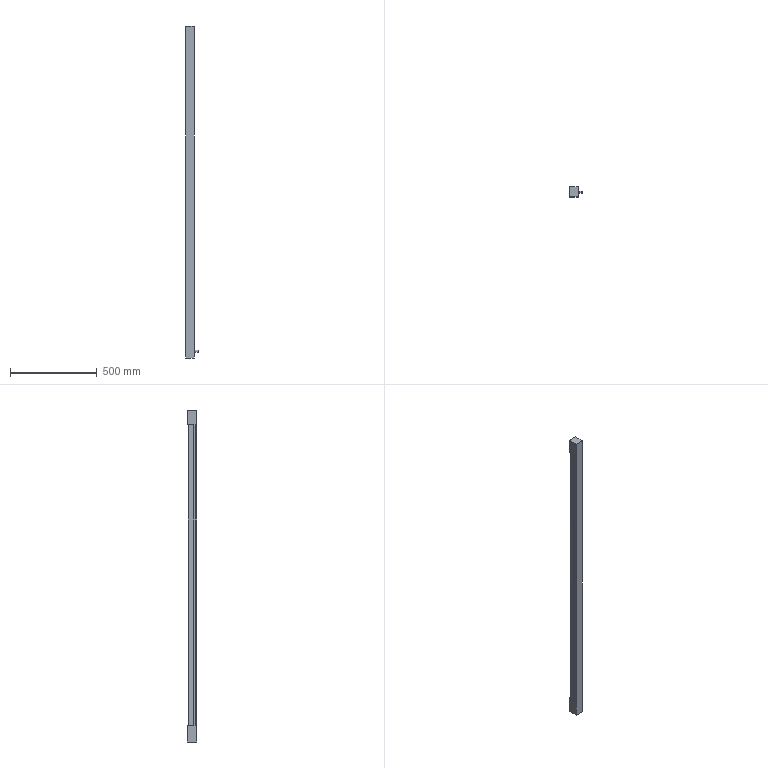Part | SolidWorks | features Boss 3, 3DProfileFeature 1, Chamfer 1, CirPattern 1, Cut 1, Extrusion 1, HoleWzd 1 | 1 solid | 74 faces | box 74.5 x 55.5 x 1910 mm | volume 4257863 mm3 | plane 44 | cylinder 20 | cone 10 | commonest cylinder face diameters 4.2 x8 5 x8 12 x2 47 x2